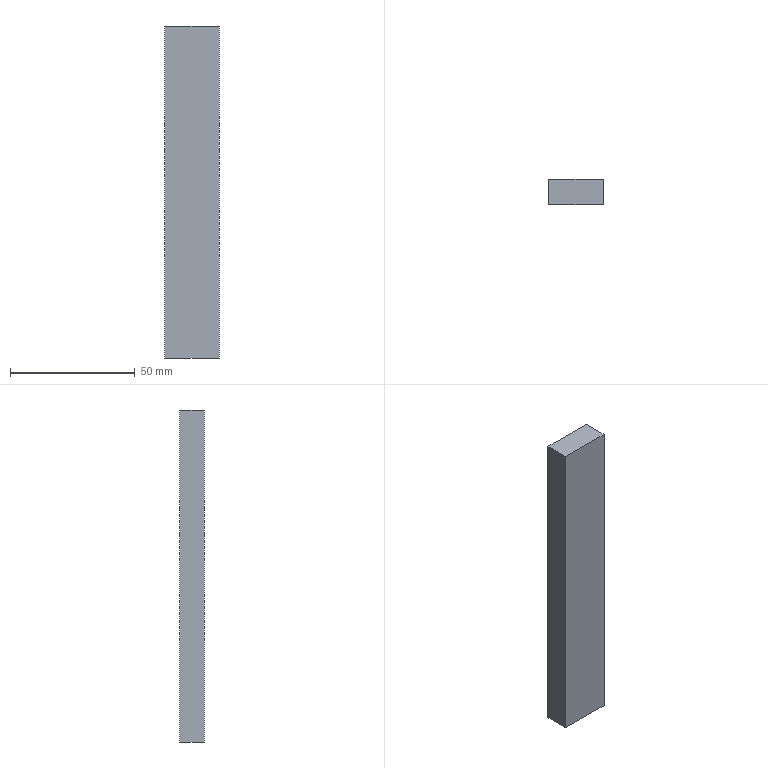Part | STEP file | 1 solid | 6 faces | box 21.772 x 10 x 133 mm | volume 28956 mm3 | plane 6
STEP:
#1=CARTESIAN_POINT('',(0.,0.,0.));
#2=DIRECTION('',(0.,0.,1.));
#3=DIRECTION('',(1.,0.,0.));
#4=AXIS2_PLACEMENT_3D('',#1,#2,#3);
#5=CARTESIAN_POINT('',(60.959,79.267,216.926));
#6=VERTEX_POINT('',#5);
#7=CARTESIAN_POINT('',(60.959,79.267,349.926));
#8=VERTEX_POINT('',#7);
#9=CARTESIAN_POINT('',(60.959,79.267,216.926));
#10=DIRECTION('',(0.,0.,1.));
#11=VECTOR('',#10,1.);
#12=LINE('',#9,#11);
#13=CARTESIAN_POINT('',(60.959,89.267,216.926));
#14=DIRECTION('',(1.,0.,0.));
#15=DIRECTION('',(0.,1.,0.));
#16=AXIS2_PLACEMENT_3D('',#13,#14,#15);
#17=PLANE('',#16);
#18=CARTESIAN_POINT('',(-10.,0.));
#19=DIRECTION('',(0.,1.));
#20=VECTOR('',#19,1.);
#21=LINE('',#18,#20);
#22=(GEOMETRIC_REPRESENTATION_CONTEXT(2)PARAMETRIC_REPRESENTATION_CONTEXT()REPRESENTATION_CONTEXT('',''));
#23=DEFINITIONAL_REPRESENTATION('',(#21),#22);
#24=PCURVE('',#17,#23);
#25=CARTESIAN_POINT('',(0.,79.267,0.));
#26=DIRECTION('',(0.,1.,0.));
#27=DIRECTION('',(0.,0.,1.));
#28=AXIS2_PLACEMENT_3D('',#25,#26,#27);
#29=PLANE('',#28);
#30=CARTESIAN_POINT('',(216.926,60.959));
#31=DIRECTION('',(1.,0.));
#32=VECTOR('',#31,1.);
#33=LINE('',#30,#32);
#34=(GEOMETRIC_REPRESENTATION_CONTEXT(2)PARAMETRIC_REPRESENTATION_CONTEXT()REPRESENTATION_CONTEXT('',''));
#35=DEFINITIONAL_REPRESENTATION('',(#33),#34);
#36=PCURVE('',#29,#35);
#37=SURFACE_CURVE('',#12,(#24,#36),.PCURVE_S1.);
#38=EDGE_CURVE('',#6,#8,#37,.T.);
#39=ORIENTED_EDGE('',*,*,#38,.T.);
#40=CARTESIAN_POINT('',(60.959,89.267,349.926));
#41=VERTEX_POINT('',#40);
#42=CARTESIAN_POINT('',(60.959,89.267,349.926));
#43=DIRECTION('',(0.,-1.,0.));
#44=VECTOR('',#43,1.);
#45=LINE('',#42,#44);
#46=CARTESIAN_POINT('',(0.,133.));
#47=DIRECTION('',(-1.,0.));
#48=VECTOR('',#47,1.);
#49=LINE('',#46,#48);
#50=(GEOMETRIC_REPRESENTATION_CONTEXT(2)PARAMETRIC_REPRESENTATION_CONTEXT()REPRESENTATION_CONTEXT('',''));
#51=DEFINITIONAL_REPRESENTATION('',(#49),#50);
#52=PCURVE('',#17,#51);
#53=CARTESIAN_POINT('',(60.959,89.267,349.926));
#54=DIRECTION('',(0.,0.,-1.));
#55=DIRECTION('',(-1.,0.,0.));
#56=AXIS2_PLACEMENT_3D('',#53,#54,#55);
#57=PLANE('',#56);
#58=CARTESIAN_POINT('',(0.,0.));
#59=DIRECTION('',(0.,-1.));
#60=VECTOR('',#59,1.);
#61=LINE('',#58,#60);
#62=(GEOMETRIC_REPRESENTATION_CONTEXT(2)PARAMETRIC_REPRESENTATION_CONTEXT()REPRESENTATION_CONTEXT('',''));
#63=DEFINITIONAL_REPRESENTATION('',(#61),#62);
#64=PCURVE('',#57,#63);
#65=SURFACE_CURVE('',#45,(#52,#64),.PCURVE_S1.);
#66=EDGE_CURVE('',#41,#8,#65,.T.);
#67=ORIENTED_EDGE('',*,*,#66,.F.);
#68=CARTESIAN_POINT('',(60.959,89.267,216.926));
#69=VERTEX_POINT('',#68);
#70=CARTESIAN_POINT('',(60.959,89.267,216.926));
#71=DIRECTION('',(0.,0.,1.));
#72=VECTOR('',#71,1.);
#73=LINE('',#70,#72);
#74=CARTESIAN_POINT('',(0.,0.));
#75=DIRECTION('',(0.,1.));
#76=VECTOR('',#75,1.);
#77=LINE('',#74,#76);
#78=(GEOMETRIC_REPRESENTATION_CONTEXT(2)PARAMETRIC_REPRESENTATION_CONTEXT()REPRESENTATION_CONTEXT('',''));
#79=DEFINITIONAL_REPRESENTATION('',(#77),#78);
#80=PCURVE('',#17,#79);
#81=CARTESIAN_POINT('',(0.,89.267,0.));
#82=DIRECTION('',(0.,1.,0.));
#83=DIRECTION('',(0.,0.,1.));
#84=AXIS2_PLACEMENT_3D('',#81,#82,#83);
#85=PLANE('',#84);
#86=CARTESIAN_POINT('',(216.926,60.959));
#87=DIRECTION('',(1.,0.));
#88=VECTOR('',#87,1.);
#89=LINE('',#86,#88);
#90=(GEOMETRIC_REPRESENTATION_CONTEXT(2)PARAMETRIC_REPRESENTATION_CONTEXT()REPRESENTATION_CONTEXT('',''));
#91=DEFINITIONAL_REPRESENTATION('',(#89),#90);
#92=PCURVE('',#85,#91);
#93=SURFACE_CURVE('',#73,(#80,#92),.PCURVE_S1.);
#94=EDGE_CURVE('',#69,#41,#93,.T.);
#95=ORIENTED_EDGE('',*,*,#94,.F.);
#96=CARTESIAN_POINT('',(60.959,89.267,216.926));
#97=DIRECTION('',(0.,-1.,0.));
#98=VECTOR('',#97,1.);
#99=LINE('',#96,#98);
#100=CARTESIAN_POINT('',(0.,0.));
#101=DIRECTION('',(-1.,0.));
#102=VECTOR('',#101,1.);
#103=LINE('',#100,#102);
#104=(GEOMETRIC_REPRESENTATION_CONTEXT(2)PARAMETRIC_REPRESENTATION_CONTEXT()REPRESENTATION_CONTEXT('',''));
#105=DEFINITIONAL_REPRESENTATION('',(#103),#104);
#106=PCURVE('',#17,#105);
#107=CARTESIAN_POINT('',(60.959,89.267,216.926));
#108=DIRECTION('',(0.,0.,1.));
#109=DIRECTION('',(1.,0.,0.));
#110=AXIS2_PLACEMENT_3D('',#107,#108,#109);
#111=PLANE('',#110);
#112=CARTESIAN_POINT('',(0.,0.));
#113=DIRECTION('',(0.,-1.));
#114=VECTOR('',#113,1.);
#115=LINE('',#112,#114);
#116=(GEOMETRIC_REPRESENTATION_CONTEXT(2)PARAMETRIC_REPRESENTATION_CONTEXT()REPRESENTATION_CONTEXT('',''));
#117=DEFINITIONAL_REPRESENTATION('',(#115),#116);
#118=PCURVE('',#111,#117);
#119=SURFACE_CURVE('',#99,(#106,#118),.PCURVE_S1.);
#120=EDGE_CURVE('',#69,#6,#119,.T.);
#121=ORIENTED_EDGE('',*,*,#120,.T.);
#122=EDGE_LOOP('',(#39,#67,#95,#121));
#123=FACE_BOUND('',#122,.T.);
#124=ADVANCED_FACE('',(#123),#17,.F.);
#125=CARTESIAN_POINT('',(82.731,79.267,349.926));
#126=VERTEX_POINT('',#125);
#127=CARTESIAN_POINT('',(60.959,79.267,349.926));
#128=DIRECTION('',(1.,0.,0.));
#129=VECTOR('',#128,1.);
#130=LINE('',#127,#129);
#131=CARTESIAN_POINT('',(0.,-10.));
#132=DIRECTION('',(-1.,0.));
#133=VECTOR('',#132,1.);
#134=LINE('',#131,#133);
#135=(GEOMETRIC_REPRESENTATION_CONTEXT(2)PARAMETRIC_REPRESENTATION_CONTEXT()REPRESENTATION_CONTEXT('',''));
#136=DEFINITIONAL_REPRESENTATION('',(#134),#135);
#137=PCURVE('',#57,#136);
#138=CARTESIAN_POINT('',(349.926,60.959));
#139=DIRECTION('',(0.,1.));
#140=VECTOR('',#139,1.);
#141=LINE('',#138,#140);
#142=(GEOMETRIC_REPRESENTATION_CONTEXT(2)PARAMETRIC_REPRESENTATION_CONTEXT()REPRESENTATION_CONTEXT('',''));
#143=DEFINITIONAL_REPRESENTATION('',(#141),#142);
#144=PCURVE('',#29,#143);
#145=SURFACE_CURVE('',#130,(#137,#144),.PCURVE_S1.);
#146=EDGE_CURVE('',#8,#126,#145,.T.);
#147=ORIENTED_EDGE('',*,*,#146,.T.);
#148=CARTESIAN_POINT('',(82.731,89.267,349.926));
#149=VERTEX_POINT('',#148);
#150=CARTESIAN_POINT('',(82.731,89.267,349.926));
#151=DIRECTION('',(0.,-1.,0.));
#152=VECTOR('',#151,1.);
#153=LINE('',#150,#152);
#154=CARTESIAN_POINT('',(-21.772,0.));
#155=DIRECTION('',(0.,-1.));
#156=VECTOR('',#155,1.);
#157=LINE('',#154,#156);
#158=(GEOMETRIC_REPRESENTATION_CONTEXT(2)PARAMETRIC_REPRESENTATION_CONTEXT()REPRESENTATION_CONTEXT('',''));
#159=DEFINITIONAL_REPRESENTATION('',(#157),#158);
#160=PCURVE('',#57,#159);
#161=CARTESIAN_POINT('',(82.731,89.267,216.926));
#162=DIRECTION('',(-1.,0.,0.));
#163=DIRECTION('',(0.,-1.,0.));
#164=AXIS2_PLACEMENT_3D('',#161,#162,#163);
#165=PLANE('',#164);
#166=CARTESIAN_POINT('',(0.,133.));
#167=DIRECTION('',(1.,0.));
#168=VECTOR('',#167,1.);
#169=LINE('',#166,#168);
#170=(GEOMETRIC_REPRESENTATION_CONTEXT(2)PARAMETRIC_REPRESENTATION_CONTEXT()REPRESENTATION_CONTEXT('',''));
#171=DEFINITIONAL_REPRESENTATION('',(#169),#170);
#172=PCURVE('',#165,#171);
#173=SURFACE_CURVE('',#153,(#160,#172),.PCURVE_S1.);
#174=EDGE_CURVE('',#149,#126,#173,.T.);
#175=ORIENTED_EDGE('',*,*,#174,.F.);
#176=CARTESIAN_POINT('',(60.959,89.267,349.926));
#177=DIRECTION('',(1.,0.,0.));
#178=VECTOR('',#177,1.);
#179=LINE('',#176,#178);
#180=CARTESIAN_POINT('',(0.,0.));
#181=DIRECTION('',(-1.,0.));
#182=VECTOR('',#181,1.);
#183=LINE('',#180,#182);
#184=(GEOMETRIC_REPRESENTATION_CONTEXT(2)PARAMETRIC_REPRESENTATION_CONTEXT()REPRESENTATION_CONTEXT('',''));
#185=DEFINITIONAL_REPRESENTATION('',(#183),#184);
#186=PCURVE('',#57,#185);
#187=CARTESIAN_POINT('',(349.926,60.959));
#188=DIRECTION('',(0.,1.));
#189=VECTOR('',#188,1.);
#190=LINE('',#187,#189);
#191=(GEOMETRIC_REPRESENTATION_CONTEXT(2)PARAMETRIC_REPRESENTATION_CONTEXT()REPRESENTATION_CONTEXT('',''));
#192=DEFINITIONAL_REPRESENTATION('',(#190),#191);
#193=PCURVE('',#85,#192);
#194=SURFACE_CURVE('',#179,(#186,#193),.PCURVE_S1.);
#195=EDGE_CURVE('',#41,#149,#194,.T.);
#196=ORIENTED_EDGE('',*,*,#195,.F.);
#197=ORIENTED_EDGE('',*,*,#66,.T.);
#198=EDGE_LOOP('',(#147,#175,#196,#197));
#199=FACE_BOUND('',#198,.T.);
#200=ADVANCED_FACE('',(#199),#57,.F.);
#201=CARTESIAN_POINT('',(82.731,79.267,216.926));
#202=VERTEX_POINT('',#201);
#203=CARTESIAN_POINT('',(82.731,79.267,216.926));
#204=DIRECTION('',(0.,0.,-1.));
#205=VECTOR('',#204,1.);
#206=LINE('',#203,#205);
#207=CARTESIAN_POINT('',(10.,0.));
#208=DIRECTION('',(0.,-1.));
#209=VECTOR('',#208,1.);
#210=LINE('',#207,#209);
#211=(GEOMETRIC_REPRESENTATION_CONTEXT(2)PARAMETRIC_REPRESENTATION_CONTEXT()REPRESENTATION_CONTEXT('',''));
#212=DEFINITIONAL_REPRESENTATION('',(#210),#211);
#213=PCURVE('',#165,#212);
#214=CARTESIAN_POINT('',(216.926,82.731));
#215=DIRECTION('',(-1.,0.));
#216=VECTOR('',#215,1.);
#217=LINE('',#214,#216);
#218=(GEOMETRIC_REPRESENTATION_CONTEXT(2)PARAMETRIC_REPRESENTATION_CONTEXT()REPRESENTATION_CONTEXT('',''));
#219=DEFINITIONAL_REPRESENTATION('',(#217),#218);
#220=PCURVE('',#29,#219);
#221=SURFACE_CURVE('',#206,(#213,#220),.PCURVE_S1.);
#222=EDGE_CURVE('',#126,#202,#221,.T.);
#223=ORIENTED_EDGE('',*,*,#222,.T.);
#224=CARTESIAN_POINT('',(82.731,89.267,216.926));
#225=VERTEX_POINT('',#224);
#226=CARTESIAN_POINT('',(82.731,89.267,216.926));
#227=DIRECTION('',(0.,-1.,0.));
#228=VECTOR('',#227,1.);
#229=LINE('',#226,#228);
#230=CARTESIAN_POINT('',(0.,0.));
#231=DIRECTION('',(1.,0.));
#232=VECTOR('',#231,1.);
#233=LINE('',#230,#232);
#234=(GEOMETRIC_REPRESENTATION_CONTEXT(2)PARAMETRIC_REPRESENTATION_CONTEXT()REPRESENTATION_CONTEXT('',''));
#235=DEFINITIONAL_REPRESENTATION('',(#233),#234);
#236=PCURVE('',#165,#235);
#237=CARTESIAN_POINT('',(21.772,0.));
#238=DIRECTION('',(0.,-1.));
#239=VECTOR('',#238,1.);
#240=LINE('',#237,#239);
#241=(GEOMETRIC_REPRESENTATION_CONTEXT(2)PARAMETRIC_REPRESENTATION_CONTEXT()REPRESENTATION_CONTEXT('',''));
#242=DEFINITIONAL_REPRESENTATION('',(#240),#241);
#243=PCURVE('',#111,#242);
#244=SURFACE_CURVE('',#229,(#236,#243),.PCURVE_S1.);
#245=EDGE_CURVE('',#225,#202,#244,.T.);
#246=ORIENTED_EDGE('',*,*,#245,.F.);
#247=CARTESIAN_POINT('',(82.731,89.267,216.926));
#248=DIRECTION('',(0.,0.,-1.));
#249=VECTOR('',#248,1.);
#250=LINE('',#247,#249);
#251=CARTESIAN_POINT('',(0.,0.));
#252=DIRECTION('',(0.,-1.));
#253=VECTOR('',#252,1.);
#254=LINE('',#251,#253);
#255=(GEOMETRIC_REPRESENTATION_CONTEXT(2)PARAMETRIC_REPRESENTATION_CONTEXT()REPRESENTATION_CONTEXT('',''));
#256=DEFINITIONAL_REPRESENTATION('',(#254),#255);
#257=PCURVE('',#165,#256);
#258=CARTESIAN_POINT('',(216.926,82.731));
#259=DIRECTION('',(-1.,0.));
#260=VECTOR('',#259,1.);
#261=LINE('',#258,#260);
#262=(GEOMETRIC_REPRESENTATION_CONTEXT(2)PARAMETRIC_REPRESENTATION_CONTEXT()REPRESENTATION_CONTEXT('',''));
#263=DEFINITIONAL_REPRESENTATION('',(#261),#262);
#264=PCURVE('',#85,#263);
#265=SURFACE_CURVE('',#250,(#257,#264),.PCURVE_S1.);
#266=EDGE_CURVE('',#149,#225,#265,.T.);
#267=ORIENTED_EDGE('',*,*,#266,.F.);
#268=ORIENTED_EDGE('',*,*,#174,.T.);
#269=EDGE_LOOP('',(#223,#246,#267,#268));
#270=FACE_BOUND('',#269,.T.);
#271=ADVANCED_FACE('',(#270),#165,.F.);
#272=CARTESIAN_POINT('',(60.959,79.267,216.926));
#273=DIRECTION('',(-1.,0.,0.));
#274=VECTOR('',#273,1.);
#275=LINE('',#272,#274);
#276=CARTESIAN_POINT('',(0.,-10.));
#277=DIRECTION('',(-1.,0.));
#278=VECTOR('',#277,1.);
#279=LINE('',#276,#278);
#280=(GEOMETRIC_REPRESENTATION_CONTEXT(2)PARAMETRIC_REPRESENTATION_CONTEXT()REPRESENTATION_CONTEXT('',''));
#281=DEFINITIONAL_REPRESENTATION('',(#279),#280);
#282=PCURVE('',#111,#281);
#283=CARTESIAN_POINT('',(216.926,60.959));
#284=DIRECTION('',(0.,-1.));
#285=VECTOR('',#284,1.);
#286=LINE('',#283,#285);
#287=(GEOMETRIC_REPRESENTATION_CONTEXT(2)PARAMETRIC_REPRESENTATION_CONTEXT()REPRESENTATION_CONTEXT('',''));
#288=DEFINITIONAL_REPRESENTATION('',(#286),#287);
#289=PCURVE('',#29,#288);
#290=SURFACE_CURVE('',#275,(#282,#289),.PCURVE_S1.);
#291=EDGE_CURVE('',#202,#6,#290,.T.);
#292=ORIENTED_EDGE('',*,*,#291,.T.);
#293=ORIENTED_EDGE('',*,*,#120,.F.);
#294=CARTESIAN_POINT('',(60.959,89.267,216.926));
#295=DIRECTION('',(-1.,0.,0.));
#296=VECTOR('',#295,1.);
#297=LINE('',#294,#296);
#298=CARTESIAN_POINT('',(0.,0.));
#299=DIRECTION('',(-1.,0.));
#300=VECTOR('',#299,1.);
#301=LINE('',#298,#300);
#302=(GEOMETRIC_REPRESENTATION_CONTEXT(2)PARAMETRIC_REPRESENTATION_CONTEXT()REPRESENTATION_CONTEXT('',''));
#303=DEFINITIONAL_REPRESENTATION('',(#301),#302);
#304=PCURVE('',#111,#303);
#305=CARTESIAN_POINT('',(216.926,60.959));
#306=DIRECTION('',(0.,-1.));
#307=VECTOR('',#306,1.);
#308=LINE('',#305,#307);
#309=(GEOMETRIC_REPRESENTATION_CONTEXT(2)PARAMETRIC_REPRESENTATION_CONTEXT()REPRESENTATION_CONTEXT('',''));
#310=DEFINITIONAL_REPRESENTATION('',(#308),#309);
#311=PCURVE('',#85,#310);
#312=SURFACE_CURVE('',#297,(#304,#311),.PCURVE_S1.);
#313=EDGE_CURVE('',#225,#69,#312,.T.);
#314=ORIENTED_EDGE('',*,*,#313,.F.);
#315=ORIENTED_EDGE('',*,*,#245,.T.);
#316=EDGE_LOOP('',(#292,#293,#314,#315));
#317=FACE_BOUND('',#316,.T.);
#318=ADVANCED_FACE('',(#317),#111,.F.);
#319=ORIENTED_EDGE('',*,*,#94,.T.);
#320=ORIENTED_EDGE('',*,*,#195,.T.);
#321=ORIENTED_EDGE('',*,*,#266,.T.);
#322=ORIENTED_EDGE('',*,*,#313,.T.);
#323=EDGE_LOOP('',(#319,#320,#321,#322));
#324=FACE_BOUND('',#323,.T.);
#325=ADVANCED_FACE('',(#324),#85,.T.);
#326=ORIENTED_EDGE('',*,*,#38,.F.);
#327=ORIENTED_EDGE('',*,*,#291,.F.);
#328=ORIENTED_EDGE('',*,*,#222,.F.);
#329=ORIENTED_EDGE('',*,*,#146,.F.);
#330=EDGE_LOOP('',(#326,#327,#328,#329));
#331=FACE_BOUND('',#330,.T.);
#332=ADVANCED_FACE('',(#331),#29,.F.);
#333=CLOSED_SHELL('',(#124,#200,#271,#318,#325,#332));
#334=MANIFOLD_SOLID_BREP('',#333);
#335=(LENGTH_UNIT()NAMED_UNIT(*)SI_UNIT(.MILLI.,.METRE.));
#336=UNCERTAINTY_MEASURE_WITH_UNIT(LENGTH_MEASURE(0.0000001),#335,'','');
#337=(NAMED_UNIT(*)PLANE_ANGLE_UNIT()SI_UNIT($,.RADIAN.));
#338=(NAMED_UNIT(*)SI_UNIT($,.STERADIAN.)SOLID_ANGLE_UNIT());
#339=(GEOMETRIC_REPRESENTATION_CONTEXT(3)GLOBAL_UNCERTAINTY_ASSIGNED_CONTEXT((#336))GLOBAL_UNIT_ASSIGNED_CONTEXT((#335,#337,#338))REPRESENTATION_CONTEXT('',''));
#340=ADVANCED_BREP_SHAPE_REPRESENTATION('',(#4,#334),#339);